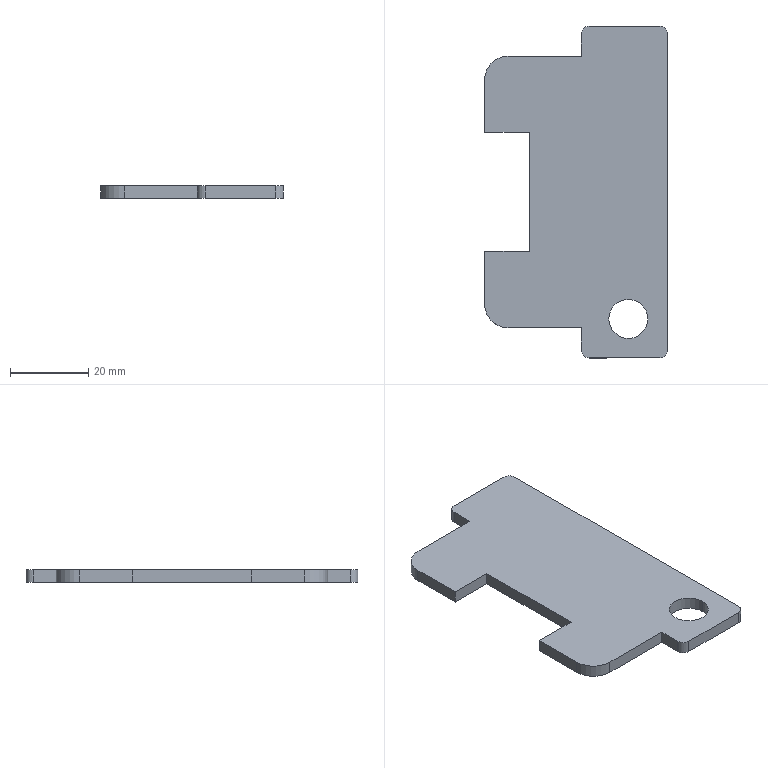Part | SolidWorks | features FlatPattern 1, SMBaseFlange 1, SheetMetal 1 | 1 solid | 22 faces | box 46.8 x 85 x 3.2 mm | volume 10065 mm3 | plane 14 | cylinder 8 | commonest cylinder face diameters 4 x4 10 x2 12 x2
STEP:
#1=CARTESIAN_POINT('',(866.02,-91.379,-3.2));
#2=VERTEX_POINT('',#1);
#3=CARTESIAN_POINT('',(876.02,-91.379,-3.2));
#4=VERTEX_POINT('',#3);
#5=CARTESIAN_POINT('',(871.02,-91.379,-3.2));
#6=DIRECTION('',(0.,0.,1.));
#7=DIRECTION('',(1.,0.,0.));
#8=AXIS2_PLACEMENT_3D('',#5,#6,#7);
#9=CIRCLE('',#8,5.);
#10=EDGE_CURVE('',#2,#4,#9,.T.);
#11=ORIENTED_EDGE('',*,*,#10,.F.);
#12=CARTESIAN_POINT('',(866.02,-91.379,0.));
#13=VERTEX_POINT('',#12);
#14=CARTESIAN_POINT('',(866.02,-91.379,-3.2));
#15=DIRECTION('',(0.,0.,1.));
#16=VECTOR('',#15,1000.);
#17=LINE('',#14,#16);
#18=EDGE_CURVE('',#2,#13,#17,.T.);
#19=ORIENTED_EDGE('',*,*,#18,.T.);
#20=CARTESIAN_POINT('',(876.02,-91.379,0.));
#21=VERTEX_POINT('',#20);
#22=CARTESIAN_POINT('',(871.02,-91.379,0.));
#23=DIRECTION('',(0.,0.,1.));
#24=DIRECTION('',(1.,0.,0.));
#25=AXIS2_PLACEMENT_3D('',#22,#23,#24);
#26=CIRCLE('',#25,5.);
#27=EDGE_CURVE('',#13,#21,#26,.T.);
#28=ORIENTED_EDGE('',*,*,#27,.T.);
#29=CARTESIAN_POINT('',(876.02,-91.379,-3.2));
#30=DIRECTION('',(0.,0.,1.));
#31=VECTOR('',#30,1000.);
#32=LINE('',#29,#31);
#33=EDGE_CURVE('',#4,#21,#32,.T.);
#34=ORIENTED_EDGE('',*,*,#33,.F.);
#35=EDGE_LOOP('',(#11,#19,#28,#34));
#36=FACE_OUTER_BOUND('',#35,.T.);
#37=CARTESIAN_POINT('',(871.02,-91.379,-3.2));
#38=DIRECTION('',(0.,0.,1.));
#39=DIRECTION('',(1.,0.,0.));
#40=AXIS2_PLACEMENT_3D('',#37,#38,#39);
#41=CYLINDRICAL_SURFACE('',#40,5.);
#42=ADVANCED_FACE('',(#36),#41,.F.);
#43=CARTESIAN_POINT('',(834.22,-30.129,0.));
#44=VERTEX_POINT('',#43);
#45=CARTESIAN_POINT('',(834.22,-43.579,0.));
#46=VERTEX_POINT('',#45);
#47=CARTESIAN_POINT('',(834.22,-43.579,0.));
#48=DIRECTION('',(0.,-1.,0.));
#49=VECTOR('',#48,1000.);
#50=LINE('',#47,#49);
#51=EDGE_CURVE('',#44,#46,#50,.T.);
#52=ORIENTED_EDGE('',*,*,#51,.F.);
#53=CARTESIAN_POINT('',(834.22,-30.129,-3.2));
#54=VERTEX_POINT('',#53);
#55=CARTESIAN_POINT('',(834.22,-30.129,-3.2));
#56=DIRECTION('',(0.,0.,1.));
#57=VECTOR('',#56,1000.);
#58=LINE('',#55,#57);
#59=EDGE_CURVE('',#54,#44,#58,.T.);
#60=ORIENTED_EDGE('',*,*,#59,.F.);
#61=CARTESIAN_POINT('',(834.22,-43.579,-3.2));
#62=VERTEX_POINT('',#61);
#63=CARTESIAN_POINT('',(834.22,-43.579,-3.2));
#64=DIRECTION('',(0.,-1.,0.));
#65=VECTOR('',#64,1000.);
#66=LINE('',#63,#65);
#67=EDGE_CURVE('',#54,#62,#66,.T.);
#68=ORIENTED_EDGE('',*,*,#67,.T.);
#69=CARTESIAN_POINT('',(834.22,-43.579,-3.2));
#70=DIRECTION('',(0.,0.,1.));
#71=VECTOR('',#70,1000.);
#72=LINE('',#69,#71);
#73=EDGE_CURVE('',#62,#46,#72,.T.);
#74=ORIENTED_EDGE('',*,*,#73,.T.);
#75=EDGE_LOOP('',(#52,#60,#68,#74));
#76=FACE_OUTER_BOUND('',#75,.T.);
#77=CARTESIAN_POINT('',(834.22,-43.579,-3.2));
#78=DIRECTION('',(-1.,0.,0.));
#79=DIRECTION('',(0.,-1.,0.));
#80=AXIS2_PLACEMENT_3D('',#77,#78,#79);
#81=PLANE('',#80);
#82=ADVANCED_FACE('',(#76),#81,.T.);
#83=CARTESIAN_POINT('',(840.22,-24.129,0.));
#84=VERTEX_POINT('',#83);
#85=CARTESIAN_POINT('',(840.22,-30.129,0.));
#86=DIRECTION('',(0.,0.,1.));
#87=DIRECTION('',(-1.,0.,0.));
#88=AXIS2_PLACEMENT_3D('',#85,#86,#87);
#89=CIRCLE('',#88,6.);
#90=EDGE_CURVE('',#84,#44,#89,.T.);
#91=ORIENTED_EDGE('',*,*,#90,.F.);
#92=CARTESIAN_POINT('',(840.22,-24.129,-3.2));
#93=VERTEX_POINT('',#92);
#94=CARTESIAN_POINT('',(840.22,-24.129,-3.2));
#95=DIRECTION('',(0.,0.,1.));
#96=VECTOR('',#95,1000.);
#97=LINE('',#94,#96);
#98=EDGE_CURVE('',#93,#84,#97,.T.);
#99=ORIENTED_EDGE('',*,*,#98,.F.);
#100=CARTESIAN_POINT('',(840.22,-30.129,-3.2));
#101=DIRECTION('',(0.,0.,1.));
#102=DIRECTION('',(-1.,0.,0.));
#103=AXIS2_PLACEMENT_3D('',#100,#101,#102);
#104=CIRCLE('',#103,6.);
#105=EDGE_CURVE('',#93,#54,#104,.T.);
#106=ORIENTED_EDGE('',*,*,#105,.T.);
#107=ORIENTED_EDGE('',*,*,#59,.T.);
#108=EDGE_LOOP('',(#91,#99,#106,#107));
#109=FACE_OUTER_BOUND('',#108,.T.);
#110=CARTESIAN_POINT('',(840.22,-30.129,-3.2));
#111=DIRECTION('',(0.,0.,1.));
#112=DIRECTION('',(1.,0.,0.));
#113=AXIS2_PLACEMENT_3D('',#110,#111,#112);
#114=CYLINDRICAL_SURFACE('',#113,6.);
#115=ADVANCED_FACE('',(#109),#114,.T.);
#116=CARTESIAN_POINT('',(859.02,-24.129,0.));
#117=VERTEX_POINT('',#116);
#118=CARTESIAN_POINT('',(840.22,-24.129,0.));
#119=DIRECTION('',(-1.,0.,0.));
#120=VECTOR('',#119,1000.);
#121=LINE('',#118,#120);
#122=EDGE_CURVE('',#117,#84,#121,.T.);
#123=ORIENTED_EDGE('',*,*,#122,.F.);
#124=CARTESIAN_POINT('',(859.02,-24.129,-3.2));
#125=VERTEX_POINT('',#124);
#126=CARTESIAN_POINT('',(859.02,-24.129,-3.2));
#127=DIRECTION('',(0.,0.,1.));
#128=VECTOR('',#127,1000.);
#129=LINE('',#126,#128);
#130=EDGE_CURVE('',#125,#117,#129,.T.);
#131=ORIENTED_EDGE('',*,*,#130,.F.);
#132=CARTESIAN_POINT('',(840.22,-24.129,-3.2));
#133=DIRECTION('',(-1.,0.,0.));
#134=VECTOR('',#133,1000.);
#135=LINE('',#132,#134);
#136=EDGE_CURVE('',#125,#93,#135,.T.);
#137=ORIENTED_EDGE('',*,*,#136,.T.);
#138=ORIENTED_EDGE('',*,*,#98,.T.);
#139=EDGE_LOOP('',(#123,#131,#137,#138));
#140=FACE_OUTER_BOUND('',#139,.T.);
#141=CARTESIAN_POINT('',(840.22,-24.129,-3.2));
#142=DIRECTION('',(0.,1.,0.));
#143=DIRECTION('',(0.,0.,1.));
#144=AXIS2_PLACEMENT_3D('',#141,#142,#143);
#145=PLANE('',#144);
#146=ADVANCED_FACE('',(#140),#145,.T.);
#147=CARTESIAN_POINT('',(859.02,-18.379,0.));
#148=VERTEX_POINT('',#147);
#149=CARTESIAN_POINT('',(859.02,-24.129,0.));
#150=DIRECTION('',(0.,-1.,0.));
#151=VECTOR('',#150,1000.);
#152=LINE('',#149,#151);
#153=EDGE_CURVE('',#148,#117,#152,.T.);
#154=ORIENTED_EDGE('',*,*,#153,.F.);
#155=CARTESIAN_POINT('',(859.02,-18.379,-3.2));
#156=VERTEX_POINT('',#155);
#157=CARTESIAN_POINT('',(859.02,-18.379,-3.2));
#158=DIRECTION('',(0.,0.,1.));
#159=VECTOR('',#158,1000.);
#160=LINE('',#157,#159);
#161=EDGE_CURVE('',#156,#148,#160,.T.);
#162=ORIENTED_EDGE('',*,*,#161,.F.);
#163=CARTESIAN_POINT('',(859.02,-24.129,-3.2));
#164=DIRECTION('',(0.,-1.,0.));
#165=VECTOR('',#164,1000.);
#166=LINE('',#163,#165);
#167=EDGE_CURVE('',#156,#125,#166,.T.);
#168=ORIENTED_EDGE('',*,*,#167,.T.);
#169=ORIENTED_EDGE('',*,*,#130,.T.);
#170=EDGE_LOOP('',(#154,#162,#168,#169));
#171=FACE_OUTER_BOUND('',#170,.T.);
#172=CARTESIAN_POINT('',(859.02,-24.129,-3.2));
#173=DIRECTION('',(-1.,0.,0.));
#174=DIRECTION('',(0.,0.,1.));
#175=AXIS2_PLACEMENT_3D('',#172,#173,#174);
#176=PLANE('',#175);
#177=ADVANCED_FACE('',(#171),#176,.T.);
#178=CARTESIAN_POINT('',(861.02,-16.379,0.));
#179=VERTEX_POINT('',#178);
#180=CARTESIAN_POINT('',(861.02,-18.379,0.));
#181=DIRECTION('',(0.,0.,1.));
#182=DIRECTION('',(-1.,0.,0.));
#183=AXIS2_PLACEMENT_3D('',#180,#181,#182);
#184=CIRCLE('',#183,2.);
#185=EDGE_CURVE('',#179,#148,#184,.T.);
#186=ORIENTED_EDGE('',*,*,#185,.F.);
#187=CARTESIAN_POINT('',(861.02,-16.379,-3.2));
#188=VERTEX_POINT('',#187);
#189=CARTESIAN_POINT('',(861.02,-16.379,-3.2));
#190=DIRECTION('',(0.,0.,1.));
#191=VECTOR('',#190,1000.);
#192=LINE('',#189,#191);
#193=EDGE_CURVE('',#188,#179,#192,.T.);
#194=ORIENTED_EDGE('',*,*,#193,.F.);
#195=CARTESIAN_POINT('',(861.02,-18.379,-3.2));
#196=DIRECTION('',(0.,0.,1.));
#197=DIRECTION('',(-1.,0.,0.));
#198=AXIS2_PLACEMENT_3D('',#195,#196,#197);
#199=CIRCLE('',#198,2.);
#200=EDGE_CURVE('',#188,#156,#199,.T.);
#201=ORIENTED_EDGE('',*,*,#200,.T.);
#202=ORIENTED_EDGE('',*,*,#161,.T.);
#203=EDGE_LOOP('',(#186,#194,#201,#202));
#204=FACE_OUTER_BOUND('',#203,.T.);
#205=CARTESIAN_POINT('',(861.02,-18.379,-3.2));
#206=DIRECTION('',(0.,0.,1.));
#207=DIRECTION('',(1.,0.,0.));
#208=AXIS2_PLACEMENT_3D('',#205,#206,#207);
#209=CYLINDRICAL_SURFACE('',#208,2.);
#210=ADVANCED_FACE('',(#204),#209,.T.);
#211=CARTESIAN_POINT('',(879.02,-16.379,0.));
#212=VERTEX_POINT('',#211);
#213=CARTESIAN_POINT('',(861.02,-16.379,0.));
#214=DIRECTION('',(-1.,0.,0.));
#215=VECTOR('',#214,1000.);
#216=LINE('',#213,#215);
#217=EDGE_CURVE('',#212,#179,#216,.T.);
#218=ORIENTED_EDGE('',*,*,#217,.F.);
#219=CARTESIAN_POINT('',(879.02,-16.379,-3.2));
#220=VERTEX_POINT('',#219);
#221=CARTESIAN_POINT('',(879.02,-16.379,-3.2));
#222=DIRECTION('',(0.,0.,1.));
#223=VECTOR('',#222,1000.);
#224=LINE('',#221,#223);
#225=EDGE_CURVE('',#220,#212,#224,.T.);
#226=ORIENTED_EDGE('',*,*,#225,.F.);
#227=CARTESIAN_POINT('',(861.02,-16.379,-3.2));
#228=DIRECTION('',(-1.,0.,0.));
#229=VECTOR('',#228,1000.);
#230=LINE('',#227,#229);
#231=EDGE_CURVE('',#220,#188,#230,.T.);
#232=ORIENTED_EDGE('',*,*,#231,.T.);
#233=ORIENTED_EDGE('',*,*,#193,.T.);
#234=EDGE_LOOP('',(#218,#226,#232,#233));
#235=FACE_OUTER_BOUND('',#234,.T.);
#236=CARTESIAN_POINT('',(861.02,-16.379,-3.2));
#237=DIRECTION('',(0.,1.,0.));
#238=DIRECTION('',(-1.,0.,0.));
#239=AXIS2_PLACEMENT_3D('',#236,#237,#238);
#240=PLANE('',#239);
#241=ADVANCED_FACE('',(#235),#240,.T.);
#242=CARTESIAN_POINT('',(881.02,-18.379,0.));
#243=VERTEX_POINT('',#242);
#244=CARTESIAN_POINT('',(879.02,-18.379,0.));
#245=DIRECTION('',(0.,0.,1.));
#246=DIRECTION('',(-1.,0.,0.));
#247=AXIS2_PLACEMENT_3D('',#244,#245,#246);
#248=CIRCLE('',#247,2.);
#249=EDGE_CURVE('',#243,#212,#248,.T.);
#250=ORIENTED_EDGE('',*,*,#249,.F.);
#251=CARTESIAN_POINT('',(881.02,-18.379,-3.2));
#252=VERTEX_POINT('',#251);
#253=CARTESIAN_POINT('',(881.02,-18.379,-3.2));
#254=DIRECTION('',(0.,0.,1.));
#255=VECTOR('',#254,1000.);
#256=LINE('',#253,#255);
#257=EDGE_CURVE('',#252,#243,#256,.T.);
#258=ORIENTED_EDGE('',*,*,#257,.F.);
#259=CARTESIAN_POINT('',(879.02,-18.379,-3.2));
#260=DIRECTION('',(0.,0.,1.));
#261=DIRECTION('',(-1.,0.,0.));
#262=AXIS2_PLACEMENT_3D('',#259,#260,#261);
#263=CIRCLE('',#262,2.);
#264=EDGE_CURVE('',#252,#220,#263,.T.);
#265=ORIENTED_EDGE('',*,*,#264,.T.);
#266=ORIENTED_EDGE('',*,*,#225,.T.);
#267=EDGE_LOOP('',(#250,#258,#265,#266));
#268=FACE_OUTER_BOUND('',#267,.T.);
#269=CARTESIAN_POINT('',(879.02,-18.379,-3.2));
#270=DIRECTION('',(0.,0.,1.));
#271=DIRECTION('',(1.,0.,0.));
#272=AXIS2_PLACEMENT_3D('',#269,#270,#271);
#273=CYLINDRICAL_SURFACE('',#272,2.);
#274=ADVANCED_FACE('',(#268),#273,.T.);
#275=CARTESIAN_POINT('',(881.02,-99.379,0.));
#276=VERTEX_POINT('',#275);
#277=CARTESIAN_POINT('',(881.02,-18.379,0.));
#278=DIRECTION('',(0.,1.,0.));
#279=VECTOR('',#278,1000.);
#280=LINE('',#277,#279);
#281=EDGE_CURVE('',#276,#243,#280,.T.);
#282=ORIENTED_EDGE('',*,*,#281,.F.);
#283=CARTESIAN_POINT('',(881.02,-99.379,-3.2));
#284=VERTEX_POINT('',#283);
#285=CARTESIAN_POINT('',(881.02,-99.379,-3.2));
#286=DIRECTION('',(0.,0.,1.));
#287=VECTOR('',#286,1000.);
#288=LINE('',#285,#287);
#289=EDGE_CURVE('',#284,#276,#288,.T.);
#290=ORIENTED_EDGE('',*,*,#289,.F.);
#291=CARTESIAN_POINT('',(881.02,-18.379,-3.2));
#292=DIRECTION('',(0.,1.,0.));
#293=VECTOR('',#292,1000.);
#294=LINE('',#291,#293);
#295=EDGE_CURVE('',#284,#252,#294,.T.);
#296=ORIENTED_EDGE('',*,*,#295,.T.);
#297=ORIENTED_EDGE('',*,*,#257,.T.);
#298=EDGE_LOOP('',(#282,#290,#296,#297));
#299=FACE_OUTER_BOUND('',#298,.T.);
#300=CARTESIAN_POINT('',(881.02,-18.379,-3.2));
#301=DIRECTION('',(1.,0.,0.));
#302=DIRECTION('',(0.,0.,-1.));
#303=AXIS2_PLACEMENT_3D('',#300,#301,#302);
#304=PLANE('',#303);
#305=ADVANCED_FACE('',(#299),#304,.T.);
#306=CARTESIAN_POINT('',(879.02,-101.379,0.));
#307=VERTEX_POINT('',#306);
#308=CARTESIAN_POINT('',(879.02,-99.379,0.));
#309=DIRECTION('',(0.,0.,1.));
#310=DIRECTION('',(-1.,0.,0.));
#311=AXIS2_PLACEMENT_3D('',#308,#309,#310);
#312=CIRCLE('',#311,2.);
#313=EDGE_CURVE('',#307,#276,#312,.T.);
#314=ORIENTED_EDGE('',*,*,#313,.F.);
#315=CARTESIAN_POINT('',(879.02,-101.379,-3.2));
#316=VERTEX_POINT('',#315);
#317=CARTESIAN_POINT('',(879.02,-101.379,-3.2));
#318=DIRECTION('',(0.,0.,1.));
#319=VECTOR('',#318,1000.);
#320=LINE('',#317,#319);
#321=EDGE_CURVE('',#316,#307,#320,.T.);
#322=ORIENTED_EDGE('',*,*,#321,.F.);
#323=CARTESIAN_POINT('',(879.02,-99.379,-3.2));
#324=DIRECTION('',(0.,0.,1.));
#325=DIRECTION('',(-1.,0.,0.));
#326=AXIS2_PLACEMENT_3D('',#323,#324,#325);
#327=CIRCLE('',#326,2.);
#328=EDGE_CURVE('',#316,#284,#327,.T.);
#329=ORIENTED_EDGE('',*,*,#328,.T.);
#330=ORIENTED_EDGE('',*,*,#289,.T.);
#331=EDGE_LOOP('',(#314,#322,#329,#330));
#332=FACE_OUTER_BOUND('',#331,.T.);
#333=CARTESIAN_POINT('',(879.02,-99.379,-3.2));
#334=DIRECTION('',(0.,0.,1.));
#335=DIRECTION('',(1.,0.,0.));
#336=AXIS2_PLACEMENT_3D('',#333,#334,#335);
#337=CYLINDRICAL_SURFACE('',#336,2.);
#338=ADVANCED_FACE('',(#332),#337,.T.);
#339=CARTESIAN_POINT('',(861.02,-101.379,0.));
#340=VERTEX_POINT('',#339);
#341=CARTESIAN_POINT('',(879.02,-101.379,0.));
#342=DIRECTION('',(1.,0.,0.));
#343=VECTOR('',#342,1000.);
#344=LINE('',#341,#343);
#345=EDGE_CURVE('',#340,#307,#344,.T.);
#346=ORIENTED_EDGE('',*,*,#345,.F.);
#347=CARTESIAN_POINT('',(861.02,-101.379,-3.2));
#348=VERTEX_POINT('',#347);
#349=CARTESIAN_POINT('',(861.02,-101.379,-3.2));
#350=DIRECTION('',(0.,0.,1.));
#351=VECTOR('',#350,1000.);
#352=LINE('',#349,#351);
#353=EDGE_CURVE('',#348,#340,#352,.T.);
#354=ORIENTED_EDGE('',*,*,#353,.F.);
#355=CARTESIAN_POINT('',(879.02,-101.379,-3.2));
#356=DIRECTION('',(1.,0.,0.));
#357=VECTOR('',#356,1000.);
#358=LINE('',#355,#357);
#359=EDGE_CURVE('',#348,#316,#358,.T.);
#360=ORIENTED_EDGE('',*,*,#359,.T.);
#361=ORIENTED_EDGE('',*,*,#321,.T.);
#362=EDGE_LOOP('',(#346,#354,#360,#361));
#363=FACE_OUTER_BOUND('',#362,.T.);
#364=CARTESIAN_POINT('',(879.02,-101.379,-3.2));
#365=DIRECTION('',(0.,-1.,0.));
#366=DIRECTION('',(1.,0.,0.));
#367=AXIS2_PLACEMENT_3D('',#364,#365,#366);
#368=PLANE('',#367);
#369=ADVANCED_FACE('',(#363),#368,.T.);
#370=CARTESIAN_POINT('',(859.02,-99.379,0.));
#371=VERTEX_POINT('',#370);
#372=CARTESIAN_POINT('',(861.02,-99.379,0.));
#373=DIRECTION('',(0.,0.,1.));
#374=DIRECTION('',(-1.,0.,0.));
#375=AXIS2_PLACEMENT_3D('',#372,#373,#374);
#376=CIRCLE('',#375,2.);
#377=EDGE_CURVE('',#371,#340,#376,.T.);
#378=ORIENTED_EDGE('',*,*,#377,.F.);
#379=CARTESIAN_POINT('',(859.02,-99.379,-3.2));
#380=VERTEX_POINT('',#379);
#381=CARTESIAN_POINT('',(859.02,-99.379,-3.2));
#382=DIRECTION('',(0.,0.,1.));
#383=VECTOR('',#382,1000.);
#384=LINE('',#381,#383);
#385=EDGE_CURVE('',#380,#371,#384,.T.);
#386=ORIENTED_EDGE('',*,*,#385,.F.);
#387=CARTESIAN_POINT('',(861.02,-99.379,-3.2));
#388=DIRECTION('',(0.,0.,1.));
#389=DIRECTION('',(-1.,0.,0.));
#390=AXIS2_PLACEMENT_3D('',#387,#388,#389);
#391=CIRCLE('',#390,2.);
#392=EDGE_CURVE('',#380,#348,#391,.T.);
#393=ORIENTED_EDGE('',*,*,#392,.T.);
#394=ORIENTED_EDGE('',*,*,#353,.T.);
#395=EDGE_LOOP('',(#378,#386,#393,#394));
#396=FACE_OUTER_BOUND('',#395,.T.);
#397=CARTESIAN_POINT('',(861.02,-99.379,-3.2));
#398=DIRECTION('',(0.,0.,1.));
#399=DIRECTION('',(1.,0.,0.));
#400=AXIS2_PLACEMENT_3D('',#397,#398,#399);
#401=CYLINDRICAL_SURFACE('',#400,2.);
#402=ADVANCED_FACE('',(#396),#401,.T.);
#403=CARTESIAN_POINT('',(859.02,-93.629,0.));
#404=VERTEX_POINT('',#403);
#405=CARTESIAN_POINT('',(859.02,-99.379,0.));
#406=DIRECTION('',(0.,-1.,0.));
#407=VECTOR('',#406,1000.);
#408=LINE('',#405,#407);
#409=EDGE_CURVE('',#404,#371,#408,.T.);
#410=ORIENTED_EDGE('',*,*,#409,.F.);
#411=CARTESIAN_POINT('',(859.02,-93.629,-3.2));
#412=VERTEX_POINT('',#411);
#413=CARTESIAN_POINT('',(859.02,-93.629,-3.2));
#414=DIRECTION('',(0.,0.,1.));
#415=VECTOR('',#414,1000.);
#416=LINE('',#413,#415);
#417=EDGE_CURVE('',#412,#404,#416,.T.);
#418=ORIENTED_EDGE('',*,*,#417,.F.);
#419=CARTESIAN_POINT('',(859.02,-99.379,-3.2));
#420=DIRECTION('',(0.,-1.,0.));
#421=VECTOR('',#420,1000.);
#422=LINE('',#419,#421);
#423=EDGE_CURVE('',#412,#380,#422,.T.);
#424=ORIENTED_EDGE('',*,*,#423,.T.);
#425=ORIENTED_EDGE('',*,*,#385,.T.);
#426=EDGE_LOOP('',(#410,#418,#424,#425));
#427=FACE_OUTER_BOUND('',#426,.T.);
#428=CARTESIAN_POINT('',(859.02,-99.379,-3.2));
#429=DIRECTION('',(-1.,0.,0.));
#430=DIRECTION('',(0.,0.,1.));
#431=AXIS2_PLACEMENT_3D('',#428,#429,#430);
#432=PLANE('',#431);
#433=ADVANCED_FACE('',(#427),#432,.T.);
#434=CARTESIAN_POINT('',(840.22,-93.629,0.));
#435=VERTEX_POINT('',#434);
#436=CARTESIAN_POINT('',(859.02,-93.629,0.));
#437=DIRECTION('',(1.,0.,0.));
#438=VECTOR('',#437,1000.);
#439=LINE('',#436,#438);
#440=EDGE_CURVE('',#435,#404,#439,.T.);
#441=ORIENTED_EDGE('',*,*,#440,.F.);
#442=CARTESIAN_POINT('',(840.22,-93.629,-3.2));
#443=VERTEX_POINT('',#442);
#444=CARTESIAN_POINT('',(840.22,-93.629,-3.2));
#445=DIRECTION('',(0.,0.,1.));
#446=VECTOR('',#445,1000.);
#447=LINE('',#444,#446);
#448=EDGE_CURVE('',#443,#435,#447,.T.);
#449=ORIENTED_EDGE('',*,*,#448,.F.);
#450=CARTESIAN_POINT('',(859.02,-93.629,-3.2));
#451=DIRECTION('',(1.,0.,0.));
#452=VECTOR('',#451,1000.);
#453=LINE('',#450,#452);
#454=EDGE_CURVE('',#443,#412,#453,.T.);
#455=ORIENTED_EDGE('',*,*,#454,.T.);
#456=ORIENTED_EDGE('',*,*,#417,.T.);
#457=EDGE_LOOP('',(#441,#449,#455,#456));
#458=FACE_OUTER_BOUND('',#457,.T.);
#459=CARTESIAN_POINT('',(859.02,-93.629,-3.2));
#460=DIRECTION('',(0.,-1.,0.));
#461=DIRECTION('',(0.,0.,-1.));
#462=AXIS2_PLACEMENT_3D('',#459,#460,#461);
#463=PLANE('',#462);
#464=ADVANCED_FACE('',(#458),#463,.T.);
#465=CARTESIAN_POINT('',(834.22,-87.629,0.));
#466=VERTEX_POINT('',#465);
#467=CARTESIAN_POINT('',(840.22,-87.629,0.));
#468=DIRECTION('',(0.,0.,1.));
#469=DIRECTION('',(1.,0.,0.));
#470=AXIS2_PLACEMENT_3D('',#467,#468,#469);
#471=CIRCLE('',#470,6.);
#472=EDGE_CURVE('',#466,#435,#471,.T.);
#473=ORIENTED_EDGE('',*,*,#472,.F.);
#474=CARTESIAN_POINT('',(834.22,-87.629,-3.2));
#475=VERTEX_POINT('',#474);
#476=CARTESIAN_POINT('',(834.22,-87.629,-3.2));
#477=DIRECTION('',(0.,0.,1.));
#478=VECTOR('',#477,1000.);
#479=LINE('',#476,#478);
#480=EDGE_CURVE('',#475,#466,#479,.T.);
#481=ORIENTED_EDGE('',*,*,#480,.F.);
#482=CARTESIAN_POINT('',(840.22,-87.629,-3.2));
#483=DIRECTION('',(0.,0.,1.));
#484=DIRECTION('',(1.,0.,0.));
#485=AXIS2_PLACEMENT_3D('',#482,#483,#484);
#486=CIRCLE('',#485,6.);
#487=EDGE_CURVE('',#475,#443,#486,.T.);
#488=ORIENTED_EDGE('',*,*,#487,.T.);
#489=ORIENTED_EDGE('',*,*,#448,.T.);
#490=EDGE_LOOP('',(#473,#481,#488,#489));
#491=FACE_OUTER_BOUND('',#490,.T.);
#492=CARTESIAN_POINT('',(840.22,-87.629,-3.2));
#493=DIRECTION('',(0.,0.,1.));
#494=DIRECTION('',(1.,0.,0.));
#495=AXIS2_PLACEMENT_3D('',#492,#493,#494);
#496=CYLINDRICAL_SURFACE('',#495,6.);
#497=ADVANCED_FACE('',(#491),#496,.T.);
#498=CARTESIAN_POINT('',(834.22,-74.079,0.));
#499=VERTEX_POINT('',#498);
#500=CARTESIAN_POINT('',(834.22,-74.079,0.));
#501=DIRECTION('',(0.,-1.,0.));
#502=VECTOR('',#501,1000.);
#503=LINE('',#500,#502);
#504=EDGE_CURVE('',#499,#466,#503,.T.);
#505=ORIENTED_EDGE('',*,*,#504,.F.);
#506=CARTESIAN_POINT('',(834.22,-74.079,-3.2));
#507=VERTEX_POINT('',#506);
#508=CARTESIAN_POINT('',(834.22,-74.079,-3.2));
#509=DIRECTION('',(0.,0.,1.));
#510=VECTOR('',#509,1000.);
#511=LINE('',#508,#510);
#512=EDGE_CURVE('',#507,#499,#511,.T.);
#513=ORIENTED_EDGE('',*,*,#512,.F.);
#514=CARTESIAN_POINT('',(834.22,-74.079,-3.2));
#515=DIRECTION('',(0.,-1.,0.));
#516=VECTOR('',#515,1000.);
#517=LINE('',#514,#516);
#518=EDGE_CURVE('',#507,#475,#517,.T.);
#519=ORIENTED_EDGE('',*,*,#518,.T.);
#520=ORIENTED_EDGE('',*,*,#480,.T.);
#521=EDGE_LOOP('',(#505,#513,#519,#520));
#522=FACE_OUTER_BOUND('',#521,.T.);
#523=CARTESIAN_POINT('',(834.22,-74.079,-3.2));
#524=DIRECTION('',(-1.,0.,0.));
#525=DIRECTION('',(0.,0.,1.));
#526=AXIS2_PLACEMENT_3D('',#523,#524,#525);
#527=PLANE('',#526);
#528=ADVANCED_FACE('',(#522),#527,.T.);
#529=CARTESIAN_POINT('',(845.72,-74.079,0.));
#530=VERTEX_POINT('',#529);
#531=CARTESIAN_POINT('',(845.72,-74.079,0.));
#532=DIRECTION('',(-1.,0.,0.));
#533=VECTOR('',#532,1000.);
#534=LINE('',#531,#533);
#535=EDGE_CURVE('',#530,#499,#534,.T.);
#536=ORIENTED_EDGE('',*,*,#535,.F.);
#537=CARTESIAN_POINT('',(845.72,-74.079,-3.2));
#538=VERTEX_POINT('',#537);
#539=CARTESIAN_POINT('',(845.72,-74.079,-3.2));
#540=DIRECTION('',(0.,0.,1.));
#541=VECTOR('',#540,1000.);
#542=LINE('',#539,#541);
#543=EDGE_CURVE('',#538,#530,#542,.T.);
#544=ORIENTED_EDGE('',*,*,#543,.F.);
#545=CARTESIAN_POINT('',(845.72,-74.079,-3.2));
#546=DIRECTION('',(-1.,0.,0.));
#547=VECTOR('',#546,1000.);
#548=LINE('',#545,#547);
#549=EDGE_CURVE('',#538,#507,#548,.T.);
#550=ORIENTED_EDGE('',*,*,#549,.T.);
#551=ORIENTED_EDGE('',*,*,#512,.T.);
#552=EDGE_LOOP('',(#536,#544,#550,#551));
#553=FACE_OUTER_BOUND('',#552,.T.);
#554=CARTESIAN_POINT('',(845.72,-74.079,-3.2));
#555=DIRECTION('',(0.,1.,0.));
#556=DIRECTION('',(0.,0.,1.));
#557=AXIS2_PLACEMENT_3D('',#554,#555,#556);
#558=PLANE('',#557);
#559=ADVANCED_FACE('',(#553),#558,.T.);
#560=CARTESIAN_POINT('',(845.72,-43.579,0.));
#561=VERTEX_POINT('',#560);
#562=CARTESIAN_POINT('',(845.72,-43.579,0.));
#563=DIRECTION('',(0.,-1.,0.));
#564=VECTOR('',#563,1000.);
#565=LINE('',#562,#564);
#566=EDGE_CURVE('',#561,#530,#565,.T.);
#567=ORIENTED_EDGE('',*,*,#566,.F.);
#568=CARTESIAN_POINT('',(845.72,-43.579,-3.2));
#569=VERTEX_POINT('',#568);
#570=CARTESIAN_POINT('',(845.72,-43.579,-3.2));
#571=DIRECTION('',(0.,0.,1.));
#572=VECTOR('',#571,1000.);
#573=LINE('',#570,#572);
#574=EDGE_CURVE('',#569,#561,#573,.T.);
#575=ORIENTED_EDGE('',*,*,#574,.F.);
#576=CARTESIAN_POINT('',(845.72,-43.579,-3.2));
#577=DIRECTION('',(0.,-1.,0.));
#578=VECTOR('',#577,1000.);
#579=LINE('',#576,#578);
#580=EDGE_CURVE('',#569,#538,#579,.T.);
#581=ORIENTED_EDGE('',*,*,#580,.T.);
#582=ORIENTED_EDGE('',*,*,#543,.T.);
#583=EDGE_LOOP('',(#567,#575,#581,#582));
#584=FACE_OUTER_BOUND('',#583,.T.);
#585=CARTESIAN_POINT('',(845.72,-43.579,-3.2));
#586=DIRECTION('',(-1.,0.,0.));
#587=DIRECTION('',(0.,0.,1.));
#588=AXIS2_PLACEMENT_3D('',#585,#586,#587);
#589=PLANE('',#588);
#590=ADVANCED_FACE('',(#584),#589,.T.);
#591=CARTESIAN_POINT('',(834.22,-43.579,0.));
#592=DIRECTION('',(1.,0.,0.));
#593=VECTOR('',#592,1000.);
#594=LINE('',#591,#593);
#595=EDGE_CURVE('',#46,#561,#594,.T.);
#596=ORIENTED_EDGE('',*,*,#595,.F.);
#597=ORIENTED_EDGE('',*,*,#73,.F.);
#598=CARTESIAN_POINT('',(834.22,-43.579,-3.2));
#599=DIRECTION('',(1.,0.,0.));
#600=VECTOR('',#599,1000.);
#601=LINE('',#598,#600);
#602=EDGE_CURVE('',#62,#569,#601,.T.);
#603=ORIENTED_EDGE('',*,*,#602,.T.);
#604=ORIENTED_EDGE('',*,*,#574,.T.);
#605=EDGE_LOOP('',(#596,#597,#603,#604));
#606=FACE_OUTER_BOUND('',#605,.T.);
#607=CARTESIAN_POINT('',(834.22,-43.579,-3.2));
#608=DIRECTION('',(0.,-1.,0.));
#609=DIRECTION('',(0.,0.,-1.));
#610=AXIS2_PLACEMENT_3D('',#607,#608,#609);
#611=PLANE('',#610);
#612=ADVANCED_FACE('',(#606),#611,.T.);
#613=CARTESIAN_POINT('',(871.02,-91.379,-3.2));
#614=DIRECTION('',(0.,0.,1.));
#615=DIRECTION('',(1.,0.,0.));
#616=AXIS2_PLACEMENT_3D('',#613,#614,#615);
#617=CIRCLE('',#616,5.);
#618=EDGE_CURVE('',#4,#2,#617,.T.);
#619=ORIENTED_EDGE('',*,*,#618,.T.);
#620=ORIENTED_EDGE('',*,*,#10,.T.);
#621=EDGE_LOOP('',(#619,#620));
#622=FACE_BOUND('',#621,.T.);
#623=ORIENTED_EDGE('',*,*,#67,.F.);
#624=ORIENTED_EDGE('',*,*,#105,.F.);
#625=ORIENTED_EDGE('',*,*,#136,.F.);
#626=ORIENTED_EDGE('',*,*,#167,.F.);
#627=ORIENTED_EDGE('',*,*,#200,.F.);
#628=ORIENTED_EDGE('',*,*,#231,.F.);
#629=ORIENTED_EDGE('',*,*,#264,.F.);
#630=ORIENTED_EDGE('',*,*,#295,.F.);
#631=ORIENTED_EDGE('',*,*,#328,.F.);
#632=ORIENTED_EDGE('',*,*,#359,.F.);
#633=ORIENTED_EDGE('',*,*,#392,.F.);
#634=ORIENTED_EDGE('',*,*,#423,.F.);
#635=ORIENTED_EDGE('',*,*,#454,.F.);
#636=ORIENTED_EDGE('',*,*,#487,.F.);
#637=ORIENTED_EDGE('',*,*,#518,.F.);
#638=ORIENTED_EDGE('',*,*,#549,.F.);
#639=ORIENTED_EDGE('',*,*,#580,.F.);
#640=ORIENTED_EDGE('',*,*,#602,.F.);
#641=EDGE_LOOP('',(#623,#624,#625,#626,#627,#628,#629,#630,#631,#632,#633,#634,#635,#636,#637,#638,#639,#640));
#642=FACE_OUTER_BOUND('',#641,.T.);
#643=CARTESIAN_POINT('',(840.22,-30.129,-3.2));
#644=DIRECTION('',(0.,0.,-1.));
#645=DIRECTION('',(-1.,0.,0.));
#646=AXIS2_PLACEMENT_3D('',#643,#644,#645);
#647=PLANE('',#646);
#648=ADVANCED_FACE('',(#622,#642),#647,.T.);
#649=CARTESIAN_POINT('',(871.02,-91.379,0.));
#650=DIRECTION('',(0.,0.,1.));
#651=DIRECTION('',(1.,0.,0.));
#652=AXIS2_PLACEMENT_3D('',#649,#650,#651);
#653=CIRCLE('',#652,5.);
#654=EDGE_CURVE('',#21,#13,#653,.T.);
#655=ORIENTED_EDGE('',*,*,#654,.F.);
#656=ORIENTED_EDGE('',*,*,#27,.F.);
#657=EDGE_LOOP('',(#655,#656));
#658=FACE_BOUND('',#657,.T.);
#659=ORIENTED_EDGE('',*,*,#51,.T.);
#660=ORIENTED_EDGE('',*,*,#595,.T.);
#661=ORIENTED_EDGE('',*,*,#566,.T.);
#662=ORIENTED_EDGE('',*,*,#535,.T.);
#663=ORIENTED_EDGE('',*,*,#504,.T.);
#664=ORIENTED_EDGE('',*,*,#472,.T.);
#665=ORIENTED_EDGE('',*,*,#440,.T.);
#666=ORIENTED_EDGE('',*,*,#409,.T.);
#667=ORIENTED_EDGE('',*,*,#377,.T.);
#668=ORIENTED_EDGE('',*,*,#345,.T.);
#669=ORIENTED_EDGE('',*,*,#313,.T.);
#670=ORIENTED_EDGE('',*,*,#281,.T.);
#671=ORIENTED_EDGE('',*,*,#249,.T.);
#672=ORIENTED_EDGE('',*,*,#217,.T.);
#673=ORIENTED_EDGE('',*,*,#185,.T.);
#674=ORIENTED_EDGE('',*,*,#153,.T.);
#675=ORIENTED_EDGE('',*,*,#122,.T.);
#676=ORIENTED_EDGE('',*,*,#90,.T.);
#677=EDGE_LOOP('',(#659,#660,#661,#662,#663,#664,#665,#666,#667,#668,#669,#670,#671,#672,#673,#674,#675,#676));
#678=FACE_OUTER_BOUND('',#677,.T.);
#679=CARTESIAN_POINT('',(840.22,-30.129,0.));
#680=DIRECTION('',(0.,0.,-1.));
#681=DIRECTION('',(-1.,0.,0.));
#682=AXIS2_PLACEMENT_3D('',#679,#680,#681);
#683=PLANE('',#682);
#684=ADVANCED_FACE('',(#658,#678),#683,.F.);
#685=ORIENTED_EDGE('',*,*,#18,.F.);
#686=ORIENTED_EDGE('',*,*,#618,.F.);
#687=ORIENTED_EDGE('',*,*,#33,.T.);
#688=ORIENTED_EDGE('',*,*,#654,.T.);
#689=EDGE_LOOP('',(#685,#686,#687,#688));
#690=FACE_OUTER_BOUND('',#689,.T.);
#691=CARTESIAN_POINT('',(871.02,-91.379,-3.2));
#692=DIRECTION('',(0.,0.,1.));
#693=DIRECTION('',(1.,0.,0.));
#694=AXIS2_PLACEMENT_3D('',#691,#692,#693);
#695=CYLINDRICAL_SURFACE('',#694,5.);
#696=ADVANCED_FACE('',(#690),#695,.F.);
#697=CLOSED_SHELL('',(#42,#82,#115,#146,#177,#210,#241,#274,#305,#338,#369,#402,#433,#464,#497,#528,#559,#590,#612,#648,#684,#696));
#698=MANIFOLD_SOLID_BREP('',#697);
#699=CARTESIAN_POINT('',(0.,0.,0.));
#700=DIRECTION('',(0.,0.,1.));
#701=DIRECTION('',(1.,0.,0.));
#702=AXIS2_PLACEMENT_3D('',#699,#700,#701);
#703=(LENGTH_UNIT()NAMED_UNIT(*)SI_UNIT(.MILLI.,.METRE.));
#704=UNCERTAINTY_MEASURE_WITH_UNIT(LENGTH_MEASURE(0.00001),#703,'','');
#705=(NAMED_UNIT(*)PLANE_ANGLE_UNIT()SI_UNIT($,.RADIAN.));
#706=(NAMED_UNIT(*)SI_UNIT($,.STERADIAN.)SOLID_ANGLE_UNIT());
#707=(GEOMETRIC_REPRESENTATION_CONTEXT(3)GLOBAL_UNCERTAINTY_ASSIGNED_CONTEXT((#704))GLOBAL_UNIT_ASSIGNED_CONTEXT((#703,#705,#706))REPRESENTATION_CONTEXT('',''));
#708=ADVANCED_BREP_SHAPE_REPRESENTATION('',(#698,#702),#707);